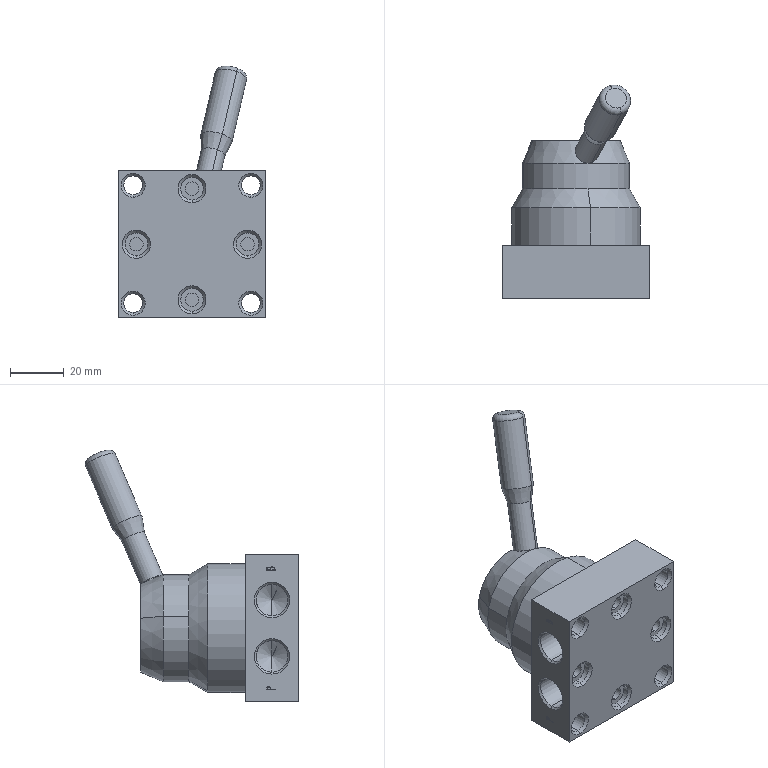Part | SolidWorks | features CompositeCurve 28, ReferencePattern 2, MirrorCompFeat 1 | 15 solids | 424 faces | box 55 x 79.723 x 94.001 mm | volume 101040 mm3 | cylinder 162 | plane 127 | cone 70 | spline 44 | torus 16 | sphere 5 | commonest cylinder face diameters 4 x25 5 x13 7 x12 11.8 x10 3 x8 3.3 x8